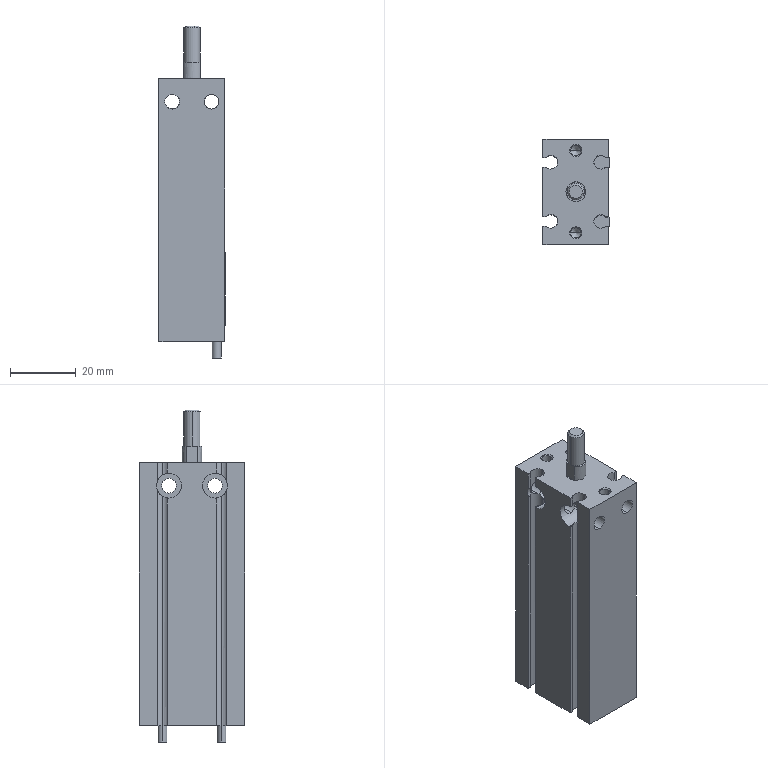Part | STEP file | CDU16-40D-A93(0) | 1 solid | 135 faces | box 20.1 x 32 x 101 mm | volume 45610 mm3 | cylinder 64 | plane 53 | cone 18 | commonest cylinder face diameters 7.6 x20 4.5 x16 4.2 x8 2.7 x4 3.14 x4 4 x4